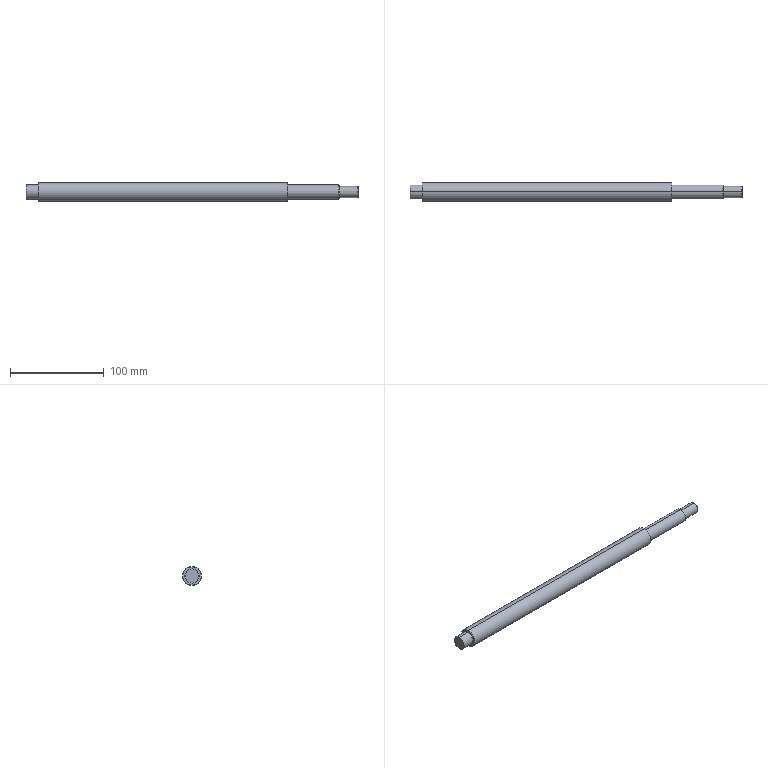Part | NX | features BREP 1 | 1 solid | 27 faces | box 354 x 20 x 20 mm | volume 97832 mm3 | cylinder 8 | torus 8 | cone 6 | plane 5 | commonest cylinder face diameters 15 x4 12 x2 20 x2
STEP:
#1=CARTESIAN_POINT('',(13.,0.,-9.7));
#2=VERTEX_POINT('',#1);
#3=CARTESIAN_POINT('',(13.3,0.,-10.));
#4=VERTEX_POINT('',#3);
#5=CARTESIAN_POINT('',(13.,0.,-9.7));
#6=DIRECTION('',(0.7071,0.,-0.7071));
#7=VECTOR('',#6,1000.);
#8=LINE('',#5,#7);
#9=EDGE_CURVE('',#2,#4,#8,.T.);
#10=ORIENTED_EDGE('',*,*,#9,.F.);
#11=CARTESIAN_POINT('',(13.,0.,9.7));
#12=VERTEX_POINT('',#11);
#13=CARTESIAN_POINT('',(13.,0.,0.));
#14=DIRECTION('',(-1.,0.,0.));
#15=DIRECTION('',(0.,0.,1.));
#16=AXIS2_PLACEMENT_3D('',#13,#14,#15);
#17=CIRCLE('',#16,9.7);
#18=EDGE_CURVE('',#12,#2,#17,.T.);
#19=ORIENTED_EDGE('',*,*,#18,.F.);
#20=CARTESIAN_POINT('',(13.3,0.,10.));
#21=VERTEX_POINT('',#20);
#22=CARTESIAN_POINT('',(13.,0.,9.7));
#23=DIRECTION('',(0.7071,0.,0.7071));
#24=VECTOR('',#23,1000.);
#25=LINE('',#22,#24);
#26=EDGE_CURVE('',#12,#21,#25,.T.);
#27=ORIENTED_EDGE('',*,*,#26,.T.);
#28=CARTESIAN_POINT('',(13.3,0.,0.));
#29=DIRECTION('',(-1.,0.,0.));
#30=DIRECTION('',(0.,0.,1.));
#31=AXIS2_PLACEMENT_3D('',#28,#29,#30);
#32=CIRCLE('',#31,10.);
#33=EDGE_CURVE('',#21,#4,#32,.T.);
#34=ORIENTED_EDGE('',*,*,#33,.T.);
#35=EDGE_LOOP('',(#10,#19,#27,#34));
#36=FACE_BOUND('',#35,.T.);
#37=CARTESIAN_POINT('',(13.15,0.,0.));
#38=DIRECTION('',(1.,0.,0.));
#39=DIRECTION('',(0.,0.,-1.));
#40=AXIS2_PLACEMENT_3D('',#37,#38,#39);
#41=CONICAL_SURFACE('',#40,9.85,0.7854);
#42=ADVANCED_FACE('',(#36),#41,.T.);
#43=CARTESIAN_POINT('',(279.,0.,10.));
#44=VERTEX_POINT('',#43);
#45=CARTESIAN_POINT('',(279.,0.,10.));
#46=DIRECTION('',(-1.,0.,0.));
#47=VECTOR('',#46,1000.);
#48=LINE('',#45,#47);
#49=EDGE_CURVE('',#21,#44,#48,.F.);
#50=ORIENTED_EDGE('',*,*,#49,.T.);
#51=CARTESIAN_POINT('',(279.,0.,-10.));
#52=VERTEX_POINT('',#51);
#53=CARTESIAN_POINT('',(279.,0.,0.));
#54=DIRECTION('',(1.,0.,0.));
#55=DIRECTION('',(0.,0.,-1.));
#56=AXIS2_PLACEMENT_3D('',#53,#54,#55);
#57=CIRCLE('',#56,10.);
#58=EDGE_CURVE('',#52,#44,#57,.T.);
#59=ORIENTED_EDGE('',*,*,#58,.F.);
#60=CARTESIAN_POINT('',(279.,0.,-10.));
#61=DIRECTION('',(-1.,0.,0.));
#62=VECTOR('',#61,1000.);
#63=LINE('',#60,#62);
#64=EDGE_CURVE('',#4,#52,#63,.F.);
#65=ORIENTED_EDGE('',*,*,#64,.F.);
#66=ORIENTED_EDGE('',*,*,#33,.F.);
#67=EDGE_LOOP('',(#50,#59,#65,#66));
#68=FACE_BOUND('',#67,.T.);
#69=CARTESIAN_POINT('',(354.,0.,0.));
#70=DIRECTION('',(-1.,0.,0.));
#71=DIRECTION('',(0.,0.,-1.));
#72=AXIS2_PLACEMENT_3D('',#69,#70,#71);
#73=CYLINDRICAL_SURFACE('',#72,10.);
#74=ADVANCED_FACE('',(#68),#73,.T.);
#75=ORIENTED_EDGE('',*,*,#64,.T.);
#76=CARTESIAN_POINT('',(279.,0.,0.));
#77=DIRECTION('',(1.,0.,0.));
#78=DIRECTION('',(0.,0.,1.));
#79=AXIS2_PLACEMENT_3D('',#76,#77,#78);
#80=CIRCLE('',#79,10.);
#81=EDGE_CURVE('',#44,#52,#80,.T.);
#82=ORIENTED_EDGE('',*,*,#81,.F.);
#83=ORIENTED_EDGE('',*,*,#49,.F.);
#84=CARTESIAN_POINT('',(13.3,0.,0.));
#85=DIRECTION('',(-1.,0.,0.));
#86=DIRECTION('',(0.,0.,-1.));
#87=AXIS2_PLACEMENT_3D('',#84,#85,#86);
#88=CIRCLE('',#87,10.);
#89=EDGE_CURVE('',#4,#21,#88,.T.);
#90=ORIENTED_EDGE('',*,*,#89,.F.);
#91=EDGE_LOOP('',(#75,#82,#83,#90));
#92=FACE_BOUND('',#91,.T.);
#93=CARTESIAN_POINT('',(354.,0.,0.));
#94=DIRECTION('',(-1.,0.,0.));
#95=DIRECTION('',(0.,0.,-1.));
#96=AXIS2_PLACEMENT_3D('',#93,#94,#95);
#97=CYLINDRICAL_SURFACE('',#96,10.);
#98=ADVANCED_FACE('',(#92),#97,.T.);
#99=ORIENTED_EDGE('',*,*,#26,.F.);
#100=CARTESIAN_POINT('',(13.,0.,0.));
#101=DIRECTION('',(-1.,0.,0.));
#102=DIRECTION('',(0.,0.,-1.));
#103=AXIS2_PLACEMENT_3D('',#100,#101,#102);
#104=CIRCLE('',#103,9.7);
#105=EDGE_CURVE('',#2,#12,#104,.T.);
#106=ORIENTED_EDGE('',*,*,#105,.F.);
#107=ORIENTED_EDGE('',*,*,#9,.T.);
#108=ORIENTED_EDGE('',*,*,#89,.T.);
#109=EDGE_LOOP('',(#99,#106,#107,#108));
#110=FACE_BOUND('',#109,.T.);
#111=CARTESIAN_POINT('',(13.15,0.,0.));
#112=DIRECTION('',(1.,0.,0.));
#113=DIRECTION('',(0.,0.,-1.));
#114=AXIS2_PLACEMENT_3D('',#111,#112,#113);
#115=CONICAL_SURFACE('',#114,9.85,0.7854);
#116=ADVANCED_FACE('',(#110),#115,.T.);
#117=ORIENTED_EDGE('',*,*,#18,.T.);
#118=ORIENTED_EDGE('',*,*,#105,.T.);
#119=EDGE_LOOP('',(#117,#118));
#120=FACE_BOUND('',#119,.T.);
#121=CARTESIAN_POINT('',(13.,0.,7.6));
#122=VERTEX_POINT('',#121);
#123=CARTESIAN_POINT('',(13.,0.,-7.6));
#124=VERTEX_POINT('',#123);
#125=CARTESIAN_POINT('',(13.,0.,0.));
#126=DIRECTION('',(1.,0.,0.));
#127=DIRECTION('',(0.,0.,1.));
#128=AXIS2_PLACEMENT_3D('',#125,#126,#127);
#129=CIRCLE('',#128,7.6);
#130=EDGE_CURVE('',#122,#124,#129,.T.);
#131=ORIENTED_EDGE('',*,*,#130,.T.);
#132=CARTESIAN_POINT('',(13.,0.,0.));
#133=DIRECTION('',(1.,0.,0.));
#134=DIRECTION('',(0.,0.,-1.));
#135=AXIS2_PLACEMENT_3D('',#132,#133,#134);
#136=CIRCLE('',#135,7.6);
#137=EDGE_CURVE('',#124,#122,#136,.T.);
#138=ORIENTED_EDGE('',*,*,#137,.T.);
#139=EDGE_LOOP('',(#131,#138));
#140=FACE_BOUND('',#139,.T.);
#141=CARTESIAN_POINT('',(13.,7.6,0.));
#142=DIRECTION('',(1.,0.,0.));
#143=DIRECTION('',(0.,1.,0.));
#144=AXIS2_PLACEMENT_3D('',#141,#142,#143);
#145=PLANE('',#144);
#146=ADVANCED_FACE('',(#120,#140),#145,.F.);
#147=CARTESIAN_POINT('',(12.971,0.,-7.529));
#148=VERTEX_POINT('',#147);
#149=CARTESIAN_POINT('',(12.9,0.,-7.6));
#150=DIRECTION('',(0.,-1.,0.));
#151=DIRECTION('',(1.,0.,0.));
#152=AXIS2_PLACEMENT_3D('',#149,#150,#151);
#153=CIRCLE('',#152,0.1);
#154=EDGE_CURVE('',#124,#148,#153,.T.);
#155=ORIENTED_EDGE('',*,*,#154,.T.);
#156=CARTESIAN_POINT('',(12.971,0.,7.529));
#157=VERTEX_POINT('',#156);
#158=CARTESIAN_POINT('',(12.971,0.,0.));
#159=DIRECTION('',(1.,0.,0.));
#160=DIRECTION('',(0.,0.,-1.));
#161=AXIS2_PLACEMENT_3D('',#158,#159,#160);
#162=CIRCLE('',#161,7.529);
#163=EDGE_CURVE('',#148,#157,#162,.T.);
#164=ORIENTED_EDGE('',*,*,#163,.T.);
#165=CARTESIAN_POINT('',(12.9,0.,7.6));
#166=DIRECTION('',(0.,1.,0.));
#167=DIRECTION('',(1.,0.,0.));
#168=AXIS2_PLACEMENT_3D('',#165,#166,#167);
#169=CIRCLE('',#168,0.1);
#170=EDGE_CURVE('',#122,#157,#169,.T.);
#171=ORIENTED_EDGE('',*,*,#170,.F.);
#172=ORIENTED_EDGE('',*,*,#137,.F.);
#173=EDGE_LOOP('',(#155,#164,#171,#172));
#174=FACE_BOUND('',#173,.T.);
#175=CARTESIAN_POINT('',(12.9,0.,0.));
#176=DIRECTION('',(1.,0.,0.));
#177=DIRECTION('',(0.,0.,-1.));
#178=AXIS2_PLACEMENT_3D('',#175,#176,#177);
#179=TOROIDAL_SURFACE('',#178,7.6,0.1);
#180=ADVANCED_FACE('',(#174),#179,.F.);
#181=ORIENTED_EDGE('',*,*,#170,.T.);
#182=CARTESIAN_POINT('',(12.971,0.,0.));
#183=DIRECTION('',(1.,0.,0.));
#184=DIRECTION('',(0.,0.,1.));
#185=AXIS2_PLACEMENT_3D('',#182,#183,#184);
#186=CIRCLE('',#185,7.529);
#187=EDGE_CURVE('',#157,#148,#186,.T.);
#188=ORIENTED_EDGE('',*,*,#187,.T.);
#189=ORIENTED_EDGE('',*,*,#154,.F.);
#190=ORIENTED_EDGE('',*,*,#130,.F.);
#191=EDGE_LOOP('',(#181,#188,#189,#190));
#192=FACE_BOUND('',#191,.T.);
#193=CARTESIAN_POINT('',(12.9,0.,0.));
#194=DIRECTION('',(1.,0.,0.));
#195=DIRECTION('',(0.,0.,-1.));
#196=AXIS2_PLACEMENT_3D('',#193,#194,#195);
#197=TOROIDAL_SURFACE('',#196,7.6,0.1);
#198=ADVANCED_FACE('',(#192),#197,.F.);
#199=CARTESIAN_POINT('',(12.9,0.,-7.5));
#200=VERTEX_POINT('',#199);
#201=CARTESIAN_POINT('',(12.9,0.,-7.6));
#202=DIRECTION('',(0.,-1.,0.));
#203=DIRECTION('',(0.7071,0.,0.7071));
#204=AXIS2_PLACEMENT_3D('',#201,#202,#203);
#205=CIRCLE('',#204,0.1);
#206=EDGE_CURVE('',#148,#200,#205,.T.);
#207=ORIENTED_EDGE('',*,*,#206,.F.);
#208=ORIENTED_EDGE('',*,*,#187,.F.);
#209=CARTESIAN_POINT('',(12.9,0.,7.5));
#210=VERTEX_POINT('',#209);
#211=CARTESIAN_POINT('',(12.9,0.,7.6));
#212=DIRECTION('',(0.,1.,0.));
#213=DIRECTION('',(0.7071,0.,-0.7071));
#214=AXIS2_PLACEMENT_3D('',#211,#212,#213);
#215=CIRCLE('',#214,0.1);
#216=EDGE_CURVE('',#157,#210,#215,.T.);
#217=ORIENTED_EDGE('',*,*,#216,.T.);
#218=CARTESIAN_POINT('',(12.9,0.,0.));
#219=DIRECTION('',(1.,0.,0.));
#220=DIRECTION('',(0.,0.,1.));
#221=AXIS2_PLACEMENT_3D('',#218,#219,#220);
#222=CIRCLE('',#221,7.5);
#223=EDGE_CURVE('',#210,#200,#222,.T.);
#224=ORIENTED_EDGE('',*,*,#223,.T.);
#225=EDGE_LOOP('',(#207,#208,#217,#224));
#226=FACE_BOUND('',#225,.T.);
#227=CARTESIAN_POINT('',(12.9,0.,0.));
#228=DIRECTION('',(1.,0.,0.));
#229=DIRECTION('',(0.,0.,-1.));
#230=AXIS2_PLACEMENT_3D('',#227,#228,#229);
#231=TOROIDAL_SURFACE('',#230,7.6,0.1);
#232=ADVANCED_FACE('',(#226),#231,.F.);
#233=CARTESIAN_POINT('',(0.,0.,-7.5));
#234=VERTEX_POINT('',#233);
#235=CARTESIAN_POINT('',(12.9,0.,-7.5));
#236=DIRECTION('',(-1.,0.,0.));
#237=VECTOR('',#236,1000.);
#238=LINE('',#235,#237);
#239=EDGE_CURVE('',#200,#234,#238,.T.);
#240=ORIENTED_EDGE('',*,*,#239,.F.);
#241=ORIENTED_EDGE('',*,*,#223,.F.);
#242=CARTESIAN_POINT('',(0.,0.,7.5));
#243=VERTEX_POINT('',#242);
#244=CARTESIAN_POINT('',(12.9,0.,7.5));
#245=DIRECTION('',(-1.,0.,0.));
#246=VECTOR('',#245,1000.);
#247=LINE('',#244,#246);
#248=EDGE_CURVE('',#210,#243,#247,.T.);
#249=ORIENTED_EDGE('',*,*,#248,.T.);
#250=CARTESIAN_POINT('',(0.,0.,0.));
#251=DIRECTION('',(-1.,0.,0.));
#252=DIRECTION('',(0.,0.,-1.));
#253=AXIS2_PLACEMENT_3D('',#250,#251,#252);
#254=CIRCLE('',#253,7.5);
#255=EDGE_CURVE('',#234,#243,#254,.T.);
#256=ORIENTED_EDGE('',*,*,#255,.F.);
#257=EDGE_LOOP('',(#240,#241,#249,#256));
#258=FACE_BOUND('',#257,.T.);
#259=CARTESIAN_POINT('',(354.,0.,0.));
#260=DIRECTION('',(-1.,0.,0.));
#261=DIRECTION('',(0.,0.,-1.));
#262=AXIS2_PLACEMENT_3D('',#259,#260,#261);
#263=CYLINDRICAL_SURFACE('',#262,7.5);
#264=ADVANCED_FACE('',(#258),#263,.T.);
#265=CARTESIAN_POINT('',(0.,0.,0.));
#266=DIRECTION('',(-1.,0.,0.));
#267=DIRECTION('',(0.,0.,1.));
#268=AXIS2_PLACEMENT_3D('',#265,#266,#267);
#269=CIRCLE('',#268,7.5);
#270=EDGE_CURVE('',#243,#234,#269,.T.);
#271=ORIENTED_EDGE('',*,*,#270,.T.);
#272=ORIENTED_EDGE('',*,*,#255,.T.);
#273=EDGE_LOOP('',(#271,#272));
#274=FACE_BOUND('',#273,.T.);
#275=CARTESIAN_POINT('',(0.,0.,0.));
#276=DIRECTION('',(1.,0.,0.));
#277=DIRECTION('',(0.,1.,0.));
#278=AXIS2_PLACEMENT_3D('',#275,#276,#277);
#279=PLANE('',#278);
#280=ADVANCED_FACE('',(#274),#279,.F.);
#281=ORIENTED_EDGE('',*,*,#248,.F.);
#282=CARTESIAN_POINT('',(12.9,0.,0.));
#283=DIRECTION('',(1.,0.,0.));
#284=DIRECTION('',(0.,0.,-1.));
#285=AXIS2_PLACEMENT_3D('',#282,#283,#284);
#286=CIRCLE('',#285,7.5);
#287=EDGE_CURVE('',#200,#210,#286,.T.);
#288=ORIENTED_EDGE('',*,*,#287,.F.);
#289=ORIENTED_EDGE('',*,*,#239,.T.);
#290=ORIENTED_EDGE('',*,*,#270,.F.);
#291=EDGE_LOOP('',(#281,#288,#289,#290));
#292=FACE_BOUND('',#291,.T.);
#293=CARTESIAN_POINT('',(354.,0.,0.));
#294=DIRECTION('',(-1.,0.,0.));
#295=DIRECTION('',(0.,0.,-1.));
#296=AXIS2_PLACEMENT_3D('',#293,#294,#295);
#297=CYLINDRICAL_SURFACE('',#296,7.5);
#298=ADVANCED_FACE('',(#292),#297,.T.);
#299=ORIENTED_EDGE('',*,*,#216,.F.);
#300=ORIENTED_EDGE('',*,*,#163,.F.);
#301=ORIENTED_EDGE('',*,*,#206,.T.);
#302=ORIENTED_EDGE('',*,*,#287,.T.);
#303=EDGE_LOOP('',(#299,#300,#301,#302));
#304=FACE_BOUND('',#303,.T.);
#305=CARTESIAN_POINT('',(12.9,0.,0.));
#306=DIRECTION('',(1.,0.,0.));
#307=DIRECTION('',(0.,0.,-1.));
#308=AXIS2_PLACEMENT_3D('',#305,#306,#307);
#309=TOROIDAL_SURFACE('',#308,7.6,0.1);
#310=ADVANCED_FACE('',(#304),#309,.F.);
#311=ORIENTED_EDGE('',*,*,#81,.T.);
#312=ORIENTED_EDGE('',*,*,#58,.T.);
#313=EDGE_LOOP('',(#311,#312));
#314=FACE_BOUND('',#313,.T.);
#315=CARTESIAN_POINT('',(279.,0.,7.6));
#316=VERTEX_POINT('',#315);
#317=CARTESIAN_POINT('',(279.,0.,-7.6));
#318=VERTEX_POINT('',#317);
#319=CARTESIAN_POINT('',(279.,0.,0.));
#320=DIRECTION('',(-1.,0.,0.));
#321=DIRECTION('',(0.,0.,1.));
#322=AXIS2_PLACEMENT_3D('',#319,#320,#321);
#323=CIRCLE('',#322,7.6);
#324=EDGE_CURVE('',#316,#318,#323,.T.);
#325=ORIENTED_EDGE('',*,*,#324,.T.);
#326=CARTESIAN_POINT('',(279.,0.,0.));
#327=DIRECTION('',(-1.,0.,0.));
#328=DIRECTION('',(0.,0.,-1.));
#329=AXIS2_PLACEMENT_3D('',#326,#327,#328);
#330=CIRCLE('',#329,7.6);
#331=EDGE_CURVE('',#318,#316,#330,.T.);
#332=ORIENTED_EDGE('',*,*,#331,.T.);
#333=EDGE_LOOP('',(#325,#332));
#334=FACE_BOUND('',#333,.T.);
#335=CARTESIAN_POINT('',(279.,10.,0.));
#336=DIRECTION('',(-1.,0.,0.));
#337=DIRECTION('',(0.,0.,1.));
#338=AXIS2_PLACEMENT_3D('',#335,#336,#337);
#339=PLANE('',#338);
#340=ADVANCED_FACE('',(#314,#334),#339,.F.);
#341=CARTESIAN_POINT('',(279.029,0.,-7.529));
#342=VERTEX_POINT('',#341);
#343=CARTESIAN_POINT('',(279.1,0.,-7.6));
#344=DIRECTION('',(0.,-1.,0.));
#345=DIRECTION('',(-0.7071,0.,0.7071));
#346=AXIS2_PLACEMENT_3D('',#343,#344,#345);
#347=CIRCLE('',#346,0.1);
#348=EDGE_CURVE('',#342,#318,#347,.T.);
#349=ORIENTED_EDGE('',*,*,#348,.F.);
#350=CARTESIAN_POINT('',(279.029,0.,7.529));
#351=VERTEX_POINT('',#350);
#352=CARTESIAN_POINT('',(279.029,0.,0.));
#353=DIRECTION('',(1.,0.,0.));
#354=DIRECTION('',(0.,0.,1.));
#355=AXIS2_PLACEMENT_3D('',#352,#353,#354);
#356=CIRCLE('',#355,7.529);
#357=EDGE_CURVE('',#351,#342,#356,.T.);
#358=ORIENTED_EDGE('',*,*,#357,.F.);
#359=CARTESIAN_POINT('',(279.1,0.,7.6));
#360=DIRECTION('',(0.,1.,0.));
#361=DIRECTION('',(-0.7071,0.,-0.7071));
#362=AXIS2_PLACEMENT_3D('',#359,#360,#361);
#363=CIRCLE('',#362,0.1);
#364=EDGE_CURVE('',#351,#316,#363,.T.);
#365=ORIENTED_EDGE('',*,*,#364,.T.);
#366=ORIENTED_EDGE('',*,*,#331,.F.);
#367=EDGE_LOOP('',(#349,#358,#365,#366));
#368=FACE_BOUND('',#367,.T.);
#369=CARTESIAN_POINT('',(279.1,0.,0.));
#370=DIRECTION('',(1.,0.,0.));
#371=DIRECTION('',(0.,0.,-1.));
#372=AXIS2_PLACEMENT_3D('',#369,#370,#371);
#373=TOROIDAL_SURFACE('',#372,7.6,0.1);
#374=ADVANCED_FACE('',(#368),#373,.F.);
#375=ORIENTED_EDGE('',*,*,#364,.F.);
#376=CARTESIAN_POINT('',(279.029,0.,0.));
#377=DIRECTION('',(1.,0.,0.));
#378=DIRECTION('',(0.,0.,-1.));
#379=AXIS2_PLACEMENT_3D('',#376,#377,#378);
#380=CIRCLE('',#379,7.529);
#381=EDGE_CURVE('',#342,#351,#380,.T.);
#382=ORIENTED_EDGE('',*,*,#381,.F.);
#383=ORIENTED_EDGE('',*,*,#348,.T.);
#384=ORIENTED_EDGE('',*,*,#324,.F.);
#385=EDGE_LOOP('',(#375,#382,#383,#384));
#386=FACE_BOUND('',#385,.T.);
#387=CARTESIAN_POINT('',(279.1,0.,0.));
#388=DIRECTION('',(1.,0.,0.));
#389=DIRECTION('',(0.,0.,-1.));
#390=AXIS2_PLACEMENT_3D('',#387,#388,#389);
#391=TOROIDAL_SURFACE('',#390,7.6,0.1);
#392=ADVANCED_FACE('',(#386),#391,.F.);
#393=CARTESIAN_POINT('',(279.1,0.,-7.5));
#394=VERTEX_POINT('',#393);
#395=CARTESIAN_POINT('',(279.1,0.,-7.6));
#396=DIRECTION('',(0.,-1.,0.));
#397=DIRECTION('',(0.,0.,1.));
#398=AXIS2_PLACEMENT_3D('',#395,#396,#397);
#399=CIRCLE('',#398,0.1);
#400=EDGE_CURVE('',#394,#342,#399,.T.);
#401=ORIENTED_EDGE('',*,*,#400,.T.);
#402=ORIENTED_EDGE('',*,*,#381,.T.);
#403=CARTESIAN_POINT('',(279.1,0.,7.5));
#404=VERTEX_POINT('',#403);
#405=CARTESIAN_POINT('',(279.1,0.,7.6));
#406=DIRECTION('',(0.,1.,0.));
#407=DIRECTION('',(0.,0.,-1.));
#408=AXIS2_PLACEMENT_3D('',#405,#406,#407);
#409=CIRCLE('',#408,0.1);
#410=EDGE_CURVE('',#404,#351,#409,.T.);
#411=ORIENTED_EDGE('',*,*,#410,.F.);
#412=CARTESIAN_POINT('',(279.1,0.,0.));
#413=DIRECTION('',(-1.,0.,0.));
#414=DIRECTION('',(0.,0.,1.));
#415=AXIS2_PLACEMENT_3D('',#412,#413,#414);
#416=CIRCLE('',#415,7.5);
#417=EDGE_CURVE('',#404,#394,#416,.T.);
#418=ORIENTED_EDGE('',*,*,#417,.T.);
#419=EDGE_LOOP('',(#401,#402,#411,#418));
#420=FACE_BOUND('',#419,.T.);
#421=CARTESIAN_POINT('',(279.1,0.,0.));
#422=DIRECTION('',(1.,0.,0.));
#423=DIRECTION('',(0.,0.,-1.));
#424=AXIS2_PLACEMENT_3D('',#421,#422,#423);
#425=TOROIDAL_SURFACE('',#424,7.6,0.1);
#426=ADVANCED_FACE('',(#420),#425,.F.);
#427=CARTESIAN_POINT('',(333.5,0.,7.5));
#428=VERTEX_POINT('',#427);
#429=CARTESIAN_POINT('',(333.5,0.,7.5));
#430=DIRECTION('',(-1.,0.,0.));
#431=VECTOR('',#430,1000.);
#432=LINE('',#429,#431);
#433=EDGE_CURVE('',#404,#428,#432,.F.);
#434=ORIENTED_EDGE('',*,*,#433,.T.);
#435=CARTESIAN_POINT('',(333.5,0.,-7.5));
#436=VERTEX_POINT('',#435);
#437=CARTESIAN_POINT('',(333.5,0.,0.));
#438=DIRECTION('',(1.,0.,0.));
#439=DIRECTION('',(0.,0.,-1.));
#440=AXIS2_PLACEMENT_3D('',#437,#438,#439);
#441=CIRCLE('',#440,7.5);
#442=EDGE_CURVE('',#436,#428,#441,.T.);
#443=ORIENTED_EDGE('',*,*,#442,.F.);
#444=CARTESIAN_POINT('',(333.5,0.,-7.5));
#445=DIRECTION('',(-1.,0.,0.));
#446=VECTOR('',#445,1000.);
#447=LINE('',#444,#446);
#448=EDGE_CURVE('',#394,#436,#447,.F.);
#449=ORIENTED_EDGE('',*,*,#448,.F.);
#450=ORIENTED_EDGE('',*,*,#417,.F.);
#451=EDGE_LOOP('',(#434,#443,#449,#450));
#452=FACE_BOUND('',#451,.T.);
#453=CARTESIAN_POINT('',(354.,0.,0.));
#454=DIRECTION('',(-1.,0.,0.));
#455=DIRECTION('',(0.,0.,-1.));
#456=AXIS2_PLACEMENT_3D('',#453,#454,#455);
#457=CYLINDRICAL_SURFACE('',#456,7.5);
#458=ADVANCED_FACE('',(#452),#457,.T.);
#459=ORIENTED_EDGE('',*,*,#448,.T.);
#460=CARTESIAN_POINT('',(333.5,0.,0.));
#461=DIRECTION('',(1.,0.,0.));
#462=DIRECTION('',(0.,0.,1.));
#463=AXIS2_PLACEMENT_3D('',#460,#461,#462);
#464=CIRCLE('',#463,7.5);
#465=EDGE_CURVE('',#428,#436,#464,.T.);
#466=ORIENTED_EDGE('',*,*,#465,.F.);
#467=ORIENTED_EDGE('',*,*,#433,.F.);
#468=CARTESIAN_POINT('',(279.1,0.,0.));
#469=DIRECTION('',(-1.,0.,0.));
#470=DIRECTION('',(0.,0.,-1.));
#471=AXIS2_PLACEMENT_3D('',#468,#469,#470);
#472=CIRCLE('',#471,7.5);
#473=EDGE_CURVE('',#394,#404,#472,.T.);
#474=ORIENTED_EDGE('',*,*,#473,.F.);
#475=EDGE_LOOP('',(#459,#466,#467,#474));
#476=FACE_BOUND('',#475,.T.);
#477=CARTESIAN_POINT('',(354.,0.,0.));
#478=DIRECTION('',(-1.,0.,0.));
#479=DIRECTION('',(0.,0.,-1.));
#480=AXIS2_PLACEMENT_3D('',#477,#478,#479);
#481=CYLINDRICAL_SURFACE('',#480,7.5);
#482=ADVANCED_FACE('',(#476),#481,.T.);
#483=ORIENTED_EDGE('',*,*,#410,.T.);
#484=ORIENTED_EDGE('',*,*,#357,.T.);
#485=ORIENTED_EDGE('',*,*,#400,.F.);
#486=ORIENTED_EDGE('',*,*,#473,.T.);
#487=EDGE_LOOP('',(#483,#484,#485,#486));
#488=FACE_BOUND('',#487,.T.);
#489=CARTESIAN_POINT('',(279.1,0.,0.));
#490=DIRECTION('',(1.,0.,0.));
#491=DIRECTION('',(0.,0.,-1.));
#492=AXIS2_PLACEMENT_3D('',#489,#490,#491);
#493=TOROIDAL_SURFACE('',#492,7.6,0.1);
#494=ADVANCED_FACE('',(#488),#493,.F.);
#495=CARTESIAN_POINT('',(334.,0.,-7.));
#496=VERTEX_POINT('',#495);
#497=CARTESIAN_POINT('',(334.,0.,-7.));
#498=DIRECTION('',(-0.7071,0.,-0.7071));
#499=VECTOR('',#498,1000.);
#500=LINE('',#497,#499);
#501=EDGE_CURVE('',#496,#436,#500,.T.);
#502=ORIENTED_EDGE('',*,*,#501,.F.);
#503=CARTESIAN_POINT('',(334.,0.,7.));
#504=VERTEX_POINT('',#503);
#505=CARTESIAN_POINT('',(334.,0.,0.));
#506=DIRECTION('',(1.,0.,0.));
#507=DIRECTION('',(0.,0.,1.));
#508=AXIS2_PLACEMENT_3D('',#505,#506,#507);
#509=CIRCLE('',#508,7.);
#510=EDGE_CURVE('',#504,#496,#509,.T.);
#511=ORIENTED_EDGE('',*,*,#510,.F.);
#512=CARTESIAN_POINT('',(334.,0.,7.));
#513=DIRECTION('',(-0.7071,0.,0.7071));
#514=VECTOR('',#513,1000.);
#515=LINE('',#512,#514);
#516=EDGE_CURVE('',#504,#428,#515,.T.);
#517=ORIENTED_EDGE('',*,*,#516,.T.);
#518=ORIENTED_EDGE('',*,*,#465,.T.);
#519=EDGE_LOOP('',(#502,#511,#517,#518));
#520=FACE_BOUND('',#519,.T.);
#521=CARTESIAN_POINT('',(333.75,0.,0.));
#522=DIRECTION('',(-1.,0.,0.));
#523=DIRECTION('',(0.,0.,1.));
#524=AXIS2_PLACEMENT_3D('',#521,#522,#523);
#525=CONICAL_SURFACE('',#524,7.25,0.7854);
#526=ADVANCED_FACE('',(#520),#525,.T.);
#527=ORIENTED_EDGE('',*,*,#516,.F.);
#528=CARTESIAN_POINT('',(334.,0.,0.));
#529=DIRECTION('',(1.,0.,0.));
#530=DIRECTION('',(0.,0.,-1.));
#531=AXIS2_PLACEMENT_3D('',#528,#529,#530);
#532=CIRCLE('',#531,7.);
#533=EDGE_CURVE('',#496,#504,#532,.T.);
#534=ORIENTED_EDGE('',*,*,#533,.F.);
#535=ORIENTED_EDGE('',*,*,#501,.T.);
#536=ORIENTED_EDGE('',*,*,#442,.T.);
#537=EDGE_LOOP('',(#527,#534,#535,#536));
#538=FACE_BOUND('',#537,.T.);
#539=CARTESIAN_POINT('',(333.75,0.,0.));
#540=DIRECTION('',(-1.,0.,0.));
#541=DIRECTION('',(0.,0.,1.));
#542=AXIS2_PLACEMENT_3D('',#539,#540,#541);
#543=CONICAL_SURFACE('',#542,7.25,0.7854);
#544=ADVANCED_FACE('',(#538),#543,.T.);
#545=ORIENTED_EDGE('',*,*,#510,.T.);
#546=ORIENTED_EDGE('',*,*,#533,.T.);
#547=EDGE_LOOP('',(#545,#546));
#548=FACE_BOUND('',#547,.T.);
#549=CARTESIAN_POINT('',(334.,0.,6.));
#550=VERTEX_POINT('',#549);
#551=CARTESIAN_POINT('',(334.,0.,-6.));
#552=VERTEX_POINT('',#551);
#553=CARTESIAN_POINT('',(334.,0.,0.));
#554=DIRECTION('',(-1.,0.,0.));
#555=DIRECTION('',(0.,0.,1.));
#556=AXIS2_PLACEMENT_3D('',#553,#554,#555);
#557=CIRCLE('',#556,6.);
#558=EDGE_CURVE('',#550,#552,#557,.T.);
#559=ORIENTED_EDGE('',*,*,#558,.T.);
#560=CARTESIAN_POINT('',(334.,0.,0.));
#561=DIRECTION('',(-1.,0.,0.));
#562=DIRECTION('',(0.,0.,-1.));
#563=AXIS2_PLACEMENT_3D('',#560,#561,#562);
#564=CIRCLE('',#563,6.);
#565=EDGE_CURVE('',#552,#550,#564,.T.);
#566=ORIENTED_EDGE('',*,*,#565,.T.);
#567=EDGE_LOOP('',(#559,#566));
#568=FACE_BOUND('',#567,.T.);
#569=CARTESIAN_POINT('',(334.,7.,0.));
#570=DIRECTION('',(-1.,0.,0.));
#571=DIRECTION('',(0.,0.,1.));
#572=AXIS2_PLACEMENT_3D('',#569,#570,#571);
#573=PLANE('',#572);
#574=ADVANCED_FACE('',(#548,#568),#573,.F.);
#575=CARTESIAN_POINT('',(353.5,0.,-6.));
#576=VERTEX_POINT('',#575);
#577=CARTESIAN_POINT('',(353.5,0.,-6.));
#578=DIRECTION('',(-1.,0.,0.));
#579=VECTOR('',#578,1000.);
#580=LINE('',#577,#579);
#581=EDGE_CURVE('',#576,#552,#580,.T.);
#582=ORIENTED_EDGE('',*,*,#581,.F.);
#583=CARTESIAN_POINT('',(353.5,0.,6.));
#584=VERTEX_POINT('',#583);
#585=CARTESIAN_POINT('',(353.5,0.,0.));
#586=DIRECTION('',(1.,0.,0.));
#587=DIRECTION('',(0.,0.,1.));
#588=AXIS2_PLACEMENT_3D('',#585,#586,#587);
#589=CIRCLE('',#588,6.);
#590=EDGE_CURVE('',#584,#576,#589,.T.);
#591=ORIENTED_EDGE('',*,*,#590,.F.);
#592=CARTESIAN_POINT('',(353.5,0.,6.));
#593=DIRECTION('',(-1.,0.,0.));
#594=VECTOR('',#593,1000.);
#595=LINE('',#592,#594);
#596=EDGE_CURVE('',#584,#550,#595,.T.);
#597=ORIENTED_EDGE('',*,*,#596,.T.);
#598=ORIENTED_EDGE('',*,*,#565,.F.);
#599=EDGE_LOOP('',(#582,#591,#597,#598));
#600=FACE_BOUND('',#599,.T.);
#601=CARTESIAN_POINT('',(354.,0.,0.));
#602=DIRECTION('',(-1.,0.,0.));
#603=DIRECTION('',(0.,0.,-1.));
#604=AXIS2_PLACEMENT_3D('',#601,#602,#603);
#605=CYLINDRICAL_SURFACE('',#604,6.);
#606=ADVANCED_FACE('',(#600),#605,.T.);
#607=ORIENTED_EDGE('',*,*,#596,.F.);
#608=CARTESIAN_POINT('',(353.5,0.,0.));
#609=DIRECTION('',(1.,0.,0.));
#610=DIRECTION('',(0.,0.,-1.));
#611=AXIS2_PLACEMENT_3D('',#608,#609,#610);
#612=CIRCLE('',#611,6.);
#613=EDGE_CURVE('',#576,#584,#612,.T.);
#614=ORIENTED_EDGE('',*,*,#613,.F.);
#615=ORIENTED_EDGE('',*,*,#581,.T.);
#616=ORIENTED_EDGE('',*,*,#558,.F.);
#617=EDGE_LOOP('',(#607,#614,#615,#616));
#618=FACE_BOUND('',#617,.T.);
#619=CARTESIAN_POINT('',(354.,0.,0.));
#620=DIRECTION('',(-1.,0.,0.));
#621=DIRECTION('',(0.,0.,-1.));
#622=AXIS2_PLACEMENT_3D('',#619,#620,#621);
#623=CYLINDRICAL_SURFACE('',#622,6.);
#624=ADVANCED_FACE('',(#618),#623,.T.);
#625=CARTESIAN_POINT('',(354.,0.,5.5));
#626=VERTEX_POINT('',#625);
#627=CARTESIAN_POINT('',(354.,0.,5.5));
#628=DIRECTION('',(-0.7071,0.,0.7071));
#629=VECTOR('',#628,1000.);
#630=LINE('',#627,#629);
#631=EDGE_CURVE('',#584,#626,#630,.F.);
#632=ORIENTED_EDGE('',*,*,#631,.T.);
#633=CARTESIAN_POINT('',(354.,0.,-5.5));
#634=VERTEX_POINT('',#633);
#635=CARTESIAN_POINT('',(354.,0.,0.));
#636=DIRECTION('',(1.,0.,0.));
#637=DIRECTION('',(0.,0.,-1.));
#638=AXIS2_PLACEMENT_3D('',#635,#636,#637);
#639=CIRCLE('',#638,5.5);
#640=EDGE_CURVE('',#634,#626,#639,.T.);
#641=ORIENTED_EDGE('',*,*,#640,.F.);
#642=CARTESIAN_POINT('',(354.,0.,-5.5));
#643=DIRECTION('',(-0.7071,0.,-0.7071));
#644=VECTOR('',#643,1000.);
#645=LINE('',#642,#644);
#646=EDGE_CURVE('',#576,#634,#645,.F.);
#647=ORIENTED_EDGE('',*,*,#646,.F.);
#648=ORIENTED_EDGE('',*,*,#613,.T.);
#649=EDGE_LOOP('',(#632,#641,#647,#648));
#650=FACE_BOUND('',#649,.T.);
#651=CARTESIAN_POINT('',(353.75,0.,0.));
#652=DIRECTION('',(-1.,0.,0.));
#653=DIRECTION('',(0.,0.,1.));
#654=AXIS2_PLACEMENT_3D('',#651,#652,#653);
#655=CONICAL_SURFACE('',#654,5.75,0.7854);
#656=ADVANCED_FACE('',(#650),#655,.T.);
#657=ORIENTED_EDGE('',*,*,#646,.T.);
#658=CARTESIAN_POINT('',(354.,0.,0.));
#659=DIRECTION('',(1.,0.,0.));
#660=DIRECTION('',(0.,0.,1.));
#661=AXIS2_PLACEMENT_3D('',#658,#659,#660);
#662=CIRCLE('',#661,5.5);
#663=EDGE_CURVE('',#626,#634,#662,.T.);
#664=ORIENTED_EDGE('',*,*,#663,.F.);
#665=ORIENTED_EDGE('',*,*,#631,.F.);
#666=ORIENTED_EDGE('',*,*,#590,.T.);
#667=EDGE_LOOP('',(#657,#664,#665,#666));
#668=FACE_BOUND('',#667,.T.);
#669=CARTESIAN_POINT('',(353.75,0.,0.));
#670=DIRECTION('',(-1.,0.,0.));
#671=DIRECTION('',(0.,0.,1.));
#672=AXIS2_PLACEMENT_3D('',#669,#670,#671);
#673=CONICAL_SURFACE('',#672,5.75,0.7854);
#674=ADVANCED_FACE('',(#668),#673,.T.);
#675=ORIENTED_EDGE('',*,*,#663,.T.);
#676=ORIENTED_EDGE('',*,*,#640,.T.);
#677=EDGE_LOOP('',(#675,#676));
#678=FACE_BOUND('',#677,.T.);
#679=CARTESIAN_POINT('',(354.,5.5,0.));
#680=DIRECTION('',(-1.,0.,0.));
#681=DIRECTION('',(0.,0.,1.));
#682=AXIS2_PLACEMENT_3D('',#679,#680,#681);
#683=PLANE('',#682);
#684=ADVANCED_FACE('',(#678),#683,.F.);
#685=CLOSED_SHELL('',(#42,#74,#98,#116,#146,#180,#198,#232,#264,#280,#298,#310,#340,#374,#392,#426,#458,#482,#494,#526,#544,#574,#606,#624,#656,#674,#684));
#686=MANIFOLD_SOLID_BREP('',#685);
#687=(LENGTH_UNIT()NAMED_UNIT(*)SI_UNIT(.MILLI.,.METRE.));
#688=UNCERTAINTY_MEASURE_WITH_UNIT(LENGTH_MEASURE(0.00001),#687,'','');
#689=(NAMED_UNIT(*)PLANE_ANGLE_UNIT()SI_UNIT($,.RADIAN.));
#690=(NAMED_UNIT(*)SI_UNIT($,.STERADIAN.)SOLID_ANGLE_UNIT());
#691=(GEOMETRIC_REPRESENTATION_CONTEXT(3)GLOBAL_UNCERTAINTY_ASSIGNED_CONTEXT((#688))GLOBAL_UNIT_ASSIGNED_CONTEXT((#687,#689,#690))REPRESENTATION_CONTEXT('',''));
#692=ADVANCED_BREP_SHAPE_REPRESENTATION('',(#686),#691);